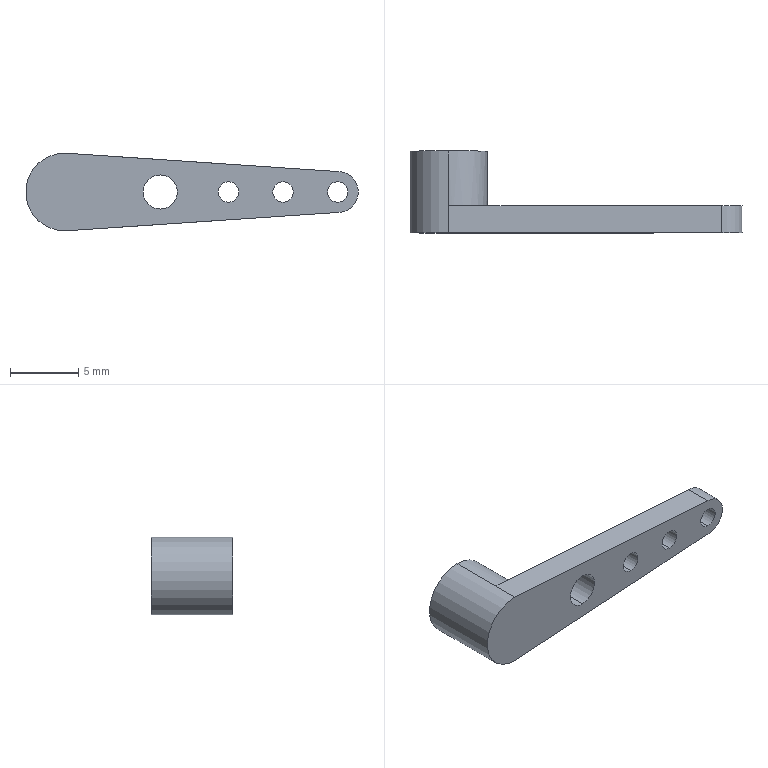Part | SolidWorks | features ICE 2, Extrusion 1 | 1 solid | 21 faces | box 24.35 x 6 x 5.701 mm | volume 238.009 mm3 | cylinder 13 | plane 8 | commonest cylinder face diameters 1.5 x6 2.5 x2 4 x2 5.701 x2 3 x1
STEP:
#1=CARTESIAN_POINT('',(20.,2.,-0.75));
#2=VERTEX_POINT('',#1);
#3=CARTESIAN_POINT('',(20.,2.,0.75));
#4=VERTEX_POINT('',#3);
#5=CARTESIAN_POINT('',(20.,2.,0.));
#6=DIRECTION('',(0.,1.,0.));
#7=DIRECTION('',(0.,0.,1.));
#8=AXIS2_PLACEMENT_3D('',#5,#6,#7);
#9=CIRCLE('',#8,0.75);
#10=EDGE_CURVE('',#2,#4,#9,.T.);
#11=ORIENTED_EDGE('',*,*,#10,.T.);
#12=CARTESIAN_POINT('',(20.,0.,0.75));
#13=VERTEX_POINT('',#12);
#14=CARTESIAN_POINT('',(20.,10.,0.75));
#15=DIRECTION('',(0.,-1.,0.));
#16=VECTOR('',#15,1000.);
#17=LINE('',#14,#16);
#18=EDGE_CURVE('',#4,#13,#17,.T.);
#19=ORIENTED_EDGE('',*,*,#18,.T.);
#20=CARTESIAN_POINT('',(20.,0.,-0.75));
#21=VERTEX_POINT('',#20);
#22=CARTESIAN_POINT('',(20.,0.,0.));
#23=DIRECTION('',(0.,-1.,0.));
#24=DIRECTION('',(0.,0.,-1.));
#25=AXIS2_PLACEMENT_3D('',#22,#23,#24);
#26=CIRCLE('',#25,0.75);
#27=EDGE_CURVE('',#13,#21,#26,.T.);
#28=ORIENTED_EDGE('',*,*,#27,.T.);
#29=CARTESIAN_POINT('',(20.,10.,-0.75));
#30=DIRECTION('',(0.,-1.,0.));
#31=VECTOR('',#30,1000.);
#32=LINE('',#29,#31);
#33=EDGE_CURVE('',#2,#21,#32,.T.);
#34=ORIENTED_EDGE('',*,*,#33,.F.);
#35=EDGE_LOOP('',(#11,#19,#28,#34));
#36=FACE_OUTER_BOUND('',#35,.T.);
#37=CARTESIAN_POINT('',(20.,10.,0.));
#38=DIRECTION('',(0.,-1.,0.));
#39=DIRECTION('',(0.,0.,-1.));
#40=AXIS2_PLACEMENT_3D('',#37,#38,#39);
#41=CYLINDRICAL_SURFACE('',#40,0.75);
#42=ADVANCED_FACE('',(#36),#41,.F.);
#43=CARTESIAN_POINT('',(7.,2.,-1.25));
#44=VERTEX_POINT('',#43);
#45=CARTESIAN_POINT('',(7.,2.,1.25));
#46=VERTEX_POINT('',#45);
#47=CARTESIAN_POINT('',(7.,2.,0.));
#48=DIRECTION('',(0.,1.,0.));
#49=DIRECTION('',(0.,0.,1.));
#50=AXIS2_PLACEMENT_3D('',#47,#48,#49);
#51=CIRCLE('',#50,1.25);
#52=EDGE_CURVE('',#44,#46,#51,.T.);
#53=ORIENTED_EDGE('',*,*,#52,.T.);
#54=CARTESIAN_POINT('',(7.,0.,1.25));
#55=VERTEX_POINT('',#54);
#56=CARTESIAN_POINT('',(7.,10.,1.25));
#57=DIRECTION('',(0.,-1.,0.));
#58=VECTOR('',#57,1000.);
#59=LINE('',#56,#58);
#60=EDGE_CURVE('',#46,#55,#59,.T.);
#61=ORIENTED_EDGE('',*,*,#60,.T.);
#62=CARTESIAN_POINT('',(7.,0.,-1.25));
#63=VERTEX_POINT('',#62);
#64=CARTESIAN_POINT('',(7.,0.,0.));
#65=DIRECTION('',(0.,-1.,0.));
#66=DIRECTION('',(0.,0.,-1.));
#67=AXIS2_PLACEMENT_3D('',#64,#65,#66);
#68=CIRCLE('',#67,1.25);
#69=EDGE_CURVE('',#55,#63,#68,.T.);
#70=ORIENTED_EDGE('',*,*,#69,.T.);
#71=CARTESIAN_POINT('',(7.,10.,-1.25));
#72=DIRECTION('',(0.,-1.,0.));
#73=VECTOR('',#72,1000.);
#74=LINE('',#71,#73);
#75=EDGE_CURVE('',#44,#63,#74,.T.);
#76=ORIENTED_EDGE('',*,*,#75,.F.);
#77=EDGE_LOOP('',(#53,#61,#70,#76));
#78=FACE_OUTER_BOUND('',#77,.T.);
#79=CARTESIAN_POINT('',(7.,10.,0.));
#80=DIRECTION('',(0.,-1.,0.));
#81=DIRECTION('',(0.,0.,-1.));
#82=AXIS2_PLACEMENT_3D('',#79,#80,#81);
#83=CYLINDRICAL_SURFACE('',#82,1.25);
#84=ADVANCED_FACE('',(#78),#83,.F.);
#85=CARTESIAN_POINT('',(12.,2.,-0.75));
#86=VERTEX_POINT('',#85);
#87=CARTESIAN_POINT('',(12.,2.,0.75));
#88=VERTEX_POINT('',#87);
#89=CARTESIAN_POINT('',(12.,2.,0.));
#90=DIRECTION('',(0.,1.,0.));
#91=DIRECTION('',(0.,0.,1.));
#92=AXIS2_PLACEMENT_3D('',#89,#90,#91);
#93=CIRCLE('',#92,0.75);
#94=EDGE_CURVE('',#86,#88,#93,.T.);
#95=ORIENTED_EDGE('',*,*,#94,.T.);
#96=CARTESIAN_POINT('',(12.,0.,0.75));
#97=VERTEX_POINT('',#96);
#98=CARTESIAN_POINT('',(12.,10.,0.75));
#99=DIRECTION('',(0.,-1.,0.));
#100=VECTOR('',#99,1000.);
#101=LINE('',#98,#100);
#102=EDGE_CURVE('',#88,#97,#101,.T.);
#103=ORIENTED_EDGE('',*,*,#102,.T.);
#104=CARTESIAN_POINT('',(12.,0.,-0.75));
#105=VERTEX_POINT('',#104);
#106=CARTESIAN_POINT('',(12.,0.,0.));
#107=DIRECTION('',(0.,-1.,0.));
#108=DIRECTION('',(0.,0.,-1.));
#109=AXIS2_PLACEMENT_3D('',#106,#107,#108);
#110=CIRCLE('',#109,0.75);
#111=EDGE_CURVE('',#97,#105,#110,.T.);
#112=ORIENTED_EDGE('',*,*,#111,.T.);
#113=CARTESIAN_POINT('',(12.,10.,-0.75));
#114=DIRECTION('',(0.,-1.,0.));
#115=VECTOR('',#114,1000.);
#116=LINE('',#113,#115);
#117=EDGE_CURVE('',#86,#105,#116,.T.);
#118=ORIENTED_EDGE('',*,*,#117,.F.);
#119=EDGE_LOOP('',(#95,#103,#112,#118));
#120=FACE_OUTER_BOUND('',#119,.T.);
#121=CARTESIAN_POINT('',(12.,10.,0.));
#122=DIRECTION('',(0.,-1.,0.));
#123=DIRECTION('',(0.,0.,-1.));
#124=AXIS2_PLACEMENT_3D('',#121,#122,#123);
#125=CYLINDRICAL_SURFACE('',#124,0.75);
#126=ADVANCED_FACE('',(#120),#125,.F.);
#127=CARTESIAN_POINT('',(16.,2.,-0.75));
#128=VERTEX_POINT('',#127);
#129=CARTESIAN_POINT('',(16.,2.,0.75));
#130=VERTEX_POINT('',#129);
#131=CARTESIAN_POINT('',(16.,2.,0.));
#132=DIRECTION('',(0.,1.,0.));
#133=DIRECTION('',(0.,0.,1.));
#134=AXIS2_PLACEMENT_3D('',#131,#132,#133);
#135=CIRCLE('',#134,0.75);
#136=EDGE_CURVE('',#128,#130,#135,.T.);
#137=ORIENTED_EDGE('',*,*,#136,.T.);
#138=CARTESIAN_POINT('',(16.,0.,0.75));
#139=VERTEX_POINT('',#138);
#140=CARTESIAN_POINT('',(16.,10.,0.75));
#141=DIRECTION('',(0.,-1.,0.));
#142=VECTOR('',#141,1000.);
#143=LINE('',#140,#142);
#144=EDGE_CURVE('',#130,#139,#143,.T.);
#145=ORIENTED_EDGE('',*,*,#144,.T.);
#146=CARTESIAN_POINT('',(16.,0.,-0.75));
#147=VERTEX_POINT('',#146);
#148=CARTESIAN_POINT('',(16.,0.,0.));
#149=DIRECTION('',(0.,-1.,0.));
#150=DIRECTION('',(0.,0.,-1.));
#151=AXIS2_PLACEMENT_3D('',#148,#149,#150);
#152=CIRCLE('',#151,0.75);
#153=EDGE_CURVE('',#139,#147,#152,.T.);
#154=ORIENTED_EDGE('',*,*,#153,.T.);
#155=CARTESIAN_POINT('',(16.,10.,-0.75));
#156=DIRECTION('',(0.,-1.,0.));
#157=VECTOR('',#156,1000.);
#158=LINE('',#155,#157);
#159=EDGE_CURVE('',#128,#147,#158,.T.);
#160=ORIENTED_EDGE('',*,*,#159,.F.);
#161=EDGE_LOOP('',(#137,#145,#154,#160));
#162=FACE_OUTER_BOUND('',#161,.T.);
#163=CARTESIAN_POINT('',(16.,10.,0.));
#164=DIRECTION('',(0.,-1.,0.));
#165=DIRECTION('',(0.,0.,-1.));
#166=AXIS2_PLACEMENT_3D('',#163,#164,#165);
#167=CYLINDRICAL_SURFACE('',#166,0.75);
#168=ADVANCED_FACE('',(#162),#167,.F.);
#169=CARTESIAN_POINT('',(0.,6.,-2.));
#170=VERTEX_POINT('',#169);
#171=CARTESIAN_POINT('',(0.,6.,2.));
#172=VERTEX_POINT('',#171);
#173=CARTESIAN_POINT('',(0.,6.,0.));
#174=DIRECTION('',(0.,1.,0.));
#175=DIRECTION('',(0.,0.,1.));
#176=AXIS2_PLACEMENT_3D('',#173,#174,#175);
#177=CIRCLE('',#176,2.);
#178=EDGE_CURVE('',#170,#172,#177,.T.);
#179=ORIENTED_EDGE('',*,*,#178,.T.);
#180=CARTESIAN_POINT('',(0.,2.,2.));
#181=VERTEX_POINT('',#180);
#182=CARTESIAN_POINT('',(0.,6.,2.));
#183=DIRECTION('',(0.,-1.,0.));
#184=VECTOR('',#183,1000.);
#185=LINE('',#182,#184);
#186=EDGE_CURVE('',#172,#181,#185,.T.);
#187=ORIENTED_EDGE('',*,*,#186,.T.);
#188=CARTESIAN_POINT('',(0.,2.,-2.));
#189=VERTEX_POINT('',#188);
#190=CARTESIAN_POINT('',(0.,2.,0.));
#191=DIRECTION('',(0.,1.,0.));
#192=DIRECTION('',(0.,0.,1.));
#193=AXIS2_PLACEMENT_3D('',#190,#191,#192);
#194=CIRCLE('',#193,2.);
#195=EDGE_CURVE('',#189,#181,#194,.T.);
#196=ORIENTED_EDGE('',*,*,#195,.F.);
#197=CARTESIAN_POINT('',(0.,6.,-2.));
#198=DIRECTION('',(0.,-1.,0.));
#199=VECTOR('',#198,1000.);
#200=LINE('',#197,#199);
#201=EDGE_CURVE('',#170,#189,#200,.T.);
#202=ORIENTED_EDGE('',*,*,#201,.F.);
#203=EDGE_LOOP('',(#179,#187,#196,#202));
#204=FACE_OUTER_BOUND('',#203,.T.);
#205=CARTESIAN_POINT('',(0.,6.,0.));
#206=DIRECTION('',(0.,-1.,0.));
#207=DIRECTION('',(0.,0.,-1.));
#208=AXIS2_PLACEMENT_3D('',#205,#206,#207);
#209=CYLINDRICAL_SURFACE('',#208,2.);
#210=ADVANCED_FACE('',(#204),#209,.F.);
#211=CARTESIAN_POINT('',(0.,6.,2.85));
#212=VERTEX_POINT('',#211);
#213=CARTESIAN_POINT('',(0.,6.,-2.85));
#214=VERTEX_POINT('',#213);
#215=CARTESIAN_POINT('',(0.,6.,0.));
#216=DIRECTION('',(0.,1.,0.));
#217=DIRECTION('',(0.,0.,1.));
#218=AXIS2_PLACEMENT_3D('',#215,#216,#217);
#219=CIRCLE('',#218,2.85);
#220=EDGE_CURVE('',#212,#214,#219,.T.);
#221=ORIENTED_EDGE('',*,*,#220,.F.);
#222=CARTESIAN_POINT('',(0.,2.,2.85));
#223=VERTEX_POINT('',#222);
#224=CARTESIAN_POINT('',(0.,2.,2.85));
#225=DIRECTION('',(0.,-1.,0.));
#226=VECTOR('',#225,1000.);
#227=LINE('',#224,#226);
#228=EDGE_CURVE('',#212,#223,#227,.T.);
#229=ORIENTED_EDGE('',*,*,#228,.T.);
#230=CARTESIAN_POINT('',(0.3831,2.,2.824));
#231=VERTEX_POINT('',#230);
#232=CARTESIAN_POINT('',(0.,2.,0.));
#233=DIRECTION('',(0.,1.,0.));
#234=DIRECTION('',(0.,0.,1.));
#235=AXIS2_PLACEMENT_3D('',#232,#233,#234);
#236=CIRCLE('',#235,2.85);
#237=EDGE_CURVE('',#223,#231,#236,.T.);
#238=ORIENTED_EDGE('',*,*,#237,.T.);
#239=CARTESIAN_POINT('',(0.3831,2.,-2.824));
#240=VERTEX_POINT('',#239);
#241=CARTESIAN_POINT('',(0.,2.,0.));
#242=DIRECTION('',(0.,1.,0.));
#243=DIRECTION('',(0.,0.,1.));
#244=AXIS2_PLACEMENT_3D('',#241,#242,#243);
#245=CIRCLE('',#244,2.85);
#246=EDGE_CURVE('',#231,#240,#245,.T.);
#247=ORIENTED_EDGE('',*,*,#246,.T.);
#248=CARTESIAN_POINT('',(0.,2.,-2.85));
#249=VERTEX_POINT('',#248);
#250=CARTESIAN_POINT('',(0.,2.,0.));
#251=DIRECTION('',(0.,1.,0.));
#252=DIRECTION('',(0.,0.,1.));
#253=AXIS2_PLACEMENT_3D('',#250,#251,#252);
#254=CIRCLE('',#253,2.85);
#255=EDGE_CURVE('',#240,#249,#254,.T.);
#256=ORIENTED_EDGE('',*,*,#255,.T.);
#257=CARTESIAN_POINT('',(0.,2.,-2.85));
#258=DIRECTION('',(0.,-1.,0.));
#259=VECTOR('',#258,1000.);
#260=LINE('',#257,#259);
#261=EDGE_CURVE('',#214,#249,#260,.T.);
#262=ORIENTED_EDGE('',*,*,#261,.F.);
#263=EDGE_LOOP('',(#221,#229,#238,#247,#256,#262));
#264=FACE_OUTER_BOUND('',#263,.T.);
#265=CARTESIAN_POINT('',(0.,2.,0.));
#266=DIRECTION('',(0.,-1.,0.));
#267=DIRECTION('',(0.,0.,-1.));
#268=AXIS2_PLACEMENT_3D('',#265,#266,#267);
#269=CYLINDRICAL_SURFACE('',#268,2.85);
#270=ADVANCED_FACE('',(#264),#269,.T.);
#271=ORIENTED_EDGE('',*,*,#228,.F.);
#272=CARTESIAN_POINT('',(0.,6.,0.));
#273=DIRECTION('',(0.,1.,0.));
#274=DIRECTION('',(0.,0.,1.));
#275=AXIS2_PLACEMENT_3D('',#272,#273,#274);
#276=CIRCLE('',#275,2.85);
#277=EDGE_CURVE('',#214,#212,#276,.T.);
#278=ORIENTED_EDGE('',*,*,#277,.F.);
#279=ORIENTED_EDGE('',*,*,#261,.T.);
#280=CARTESIAN_POINT('',(0.,0.,-2.85));
#281=VERTEX_POINT('',#280);
#282=CARTESIAN_POINT('',(0.,2.,-2.85));
#283=DIRECTION('',(0.,-1.,0.));
#284=VECTOR('',#283,1000.);
#285=LINE('',#282,#284);
#286=EDGE_CURVE('',#249,#281,#285,.T.);
#287=ORIENTED_EDGE('',*,*,#286,.T.);
#288=CARTESIAN_POINT('',(0.,0.,2.85));
#289=VERTEX_POINT('',#288);
#290=CARTESIAN_POINT('',(0.,0.,0.));
#291=DIRECTION('',(0.,1.,0.));
#292=DIRECTION('',(0.,0.,1.));
#293=AXIS2_PLACEMENT_3D('',#290,#291,#292);
#294=CIRCLE('',#293,2.85);
#295=EDGE_CURVE('',#281,#289,#294,.T.);
#296=ORIENTED_EDGE('',*,*,#295,.T.);
#297=CARTESIAN_POINT('',(0.,2.,2.85));
#298=DIRECTION('',(0.,-1.,0.));
#299=VECTOR('',#298,1000.);
#300=LINE('',#297,#299);
#301=EDGE_CURVE('',#223,#289,#300,.T.);
#302=ORIENTED_EDGE('',*,*,#301,.F.);
#303=EDGE_LOOP('',(#271,#278,#279,#287,#296,#302));
#304=FACE_OUTER_BOUND('',#303,.T.);
#305=CARTESIAN_POINT('',(0.,2.,0.));
#306=DIRECTION('',(0.,-1.,0.));
#307=DIRECTION('',(0.,0.,-1.));
#308=AXIS2_PLACEMENT_3D('',#305,#306,#307);
#309=CYLINDRICAL_SURFACE('',#308,2.85);
#310=ADVANCED_FACE('',(#304),#309,.T.);
#311=CARTESIAN_POINT('',(20.,0.,1.5));
#312=VERTEX_POINT('',#311);
#313=CARTESIAN_POINT('',(0.,0.,2.85));
#314=DIRECTION('',(0.9977,0.,-0.06736));
#315=VECTOR('',#314,1000.);
#316=LINE('',#313,#315);
#317=EDGE_CURVE('',#289,#312,#316,.T.);
#318=ORIENTED_EDGE('',*,*,#317,.T.);
#319=CARTESIAN_POINT('',(20.,2.,1.5));
#320=VERTEX_POINT('',#319);
#321=CARTESIAN_POINT('',(20.,2.,1.5));
#322=DIRECTION('',(0.,-1.,0.));
#323=VECTOR('',#322,1000.);
#324=LINE('',#321,#323);
#325=EDGE_CURVE('',#320,#312,#324,.T.);
#326=ORIENTED_EDGE('',*,*,#325,.F.);
#327=CARTESIAN_POINT('',(0.,2.,2.85));
#328=DIRECTION('',(0.9977,0.,-0.06736));
#329=VECTOR('',#328,1000.);
#330=LINE('',#327,#329);
#331=EDGE_CURVE('',#231,#320,#330,.T.);
#332=ORIENTED_EDGE('',*,*,#331,.F.);
#333=CARTESIAN_POINT('',(0.,2.,2.85));
#334=DIRECTION('',(0.9977,0.,-0.06736));
#335=VECTOR('',#334,1000.);
#336=LINE('',#333,#335);
#337=EDGE_CURVE('',#223,#231,#336,.T.);
#338=ORIENTED_EDGE('',*,*,#337,.F.);
#339=ORIENTED_EDGE('',*,*,#301,.T.);
#340=EDGE_LOOP('',(#318,#326,#332,#338,#339));
#341=FACE_OUTER_BOUND('',#340,.T.);
#342=CARTESIAN_POINT('',(0.,2.,2.85));
#343=DIRECTION('',(-0.06736,0.,-0.9977));
#344=DIRECTION('',(-0.9977,0.,0.06736));
#345=AXIS2_PLACEMENT_3D('',#342,#343,#344);
#346=PLANE('',#345);
#347=ADVANCED_FACE('',(#341),#346,.F.);
#348=CARTESIAN_POINT('',(20.,0.,-1.5));
#349=VERTEX_POINT('',#348);
#350=CARTESIAN_POINT('',(20.,0.,0.));
#351=DIRECTION('',(0.,1.,0.));
#352=DIRECTION('',(0.,0.,1.));
#353=AXIS2_PLACEMENT_3D('',#350,#351,#352);
#354=CIRCLE('',#353,1.5);
#355=EDGE_CURVE('',#312,#349,#354,.T.);
#356=ORIENTED_EDGE('',*,*,#355,.T.);
#357=CARTESIAN_POINT('',(20.,2.,-1.5));
#358=VERTEX_POINT('',#357);
#359=CARTESIAN_POINT('',(20.,2.,-1.5));
#360=DIRECTION('',(0.,-1.,0.));
#361=VECTOR('',#360,1000.);
#362=LINE('',#359,#361);
#363=EDGE_CURVE('',#358,#349,#362,.T.);
#364=ORIENTED_EDGE('',*,*,#363,.F.);
#365=CARTESIAN_POINT('',(20.,2.,0.));
#366=DIRECTION('',(0.,1.,0.));
#367=DIRECTION('',(0.,0.,1.));
#368=AXIS2_PLACEMENT_3D('',#365,#366,#367);
#369=CIRCLE('',#368,1.5);
#370=EDGE_CURVE('',#320,#358,#369,.T.);
#371=ORIENTED_EDGE('',*,*,#370,.F.);
#372=ORIENTED_EDGE('',*,*,#325,.T.);
#373=EDGE_LOOP('',(#356,#364,#371,#372));
#374=FACE_OUTER_BOUND('',#373,.T.);
#375=CARTESIAN_POINT('',(20.,2.,0.));
#376=DIRECTION('',(0.,-1.,0.));
#377=DIRECTION('',(0.,0.,-1.));
#378=AXIS2_PLACEMENT_3D('',#375,#376,#377);
#379=CYLINDRICAL_SURFACE('',#378,1.5);
#380=ADVANCED_FACE('',(#374),#379,.T.);
#381=CARTESIAN_POINT('',(0.,0.,-2.85));
#382=DIRECTION('',(-0.9977,0.,-0.06736));
#383=VECTOR('',#382,1000.);
#384=LINE('',#381,#383);
#385=EDGE_CURVE('',#349,#281,#384,.T.);
#386=ORIENTED_EDGE('',*,*,#385,.T.);
#387=ORIENTED_EDGE('',*,*,#286,.F.);
#388=CARTESIAN_POINT('',(0.,2.,-2.85));
#389=DIRECTION('',(-0.9977,0.,-0.06736));
#390=VECTOR('',#389,1000.);
#391=LINE('',#388,#390);
#392=EDGE_CURVE('',#240,#249,#391,.T.);
#393=ORIENTED_EDGE('',*,*,#392,.F.);
#394=CARTESIAN_POINT('',(0.,2.,-2.85));
#395=DIRECTION('',(-0.9977,0.,-0.06736));
#396=VECTOR('',#395,1000.);
#397=LINE('',#394,#396);
#398=EDGE_CURVE('',#358,#240,#397,.T.);
#399=ORIENTED_EDGE('',*,*,#398,.F.);
#400=ORIENTED_EDGE('',*,*,#363,.T.);
#401=EDGE_LOOP('',(#386,#387,#393,#399,#400));
#402=FACE_OUTER_BOUND('',#401,.T.);
#403=CARTESIAN_POINT('',(0.,2.,-2.85));
#404=DIRECTION('',(-0.06736,0.,0.9977));
#405=DIRECTION('',(0.9977,0.,0.06736));
#406=AXIS2_PLACEMENT_3D('',#403,#404,#405);
#407=PLANE('',#406);
#408=ADVANCED_FACE('',(#402),#407,.F.);
#409=ORIENTED_EDGE('',*,*,#10,.F.);
#410=CARTESIAN_POINT('',(20.,2.,0.));
#411=DIRECTION('',(0.,1.,0.));
#412=DIRECTION('',(0.,0.,1.));
#413=AXIS2_PLACEMENT_3D('',#410,#411,#412);
#414=CIRCLE('',#413,0.75);
#415=EDGE_CURVE('',#4,#2,#414,.T.);
#416=ORIENTED_EDGE('',*,*,#415,.F.);
#417=EDGE_LOOP('',(#409,#416));
#418=FACE_BOUND('',#417,.T.);
#419=ORIENTED_EDGE('',*,*,#52,.F.);
#420=CARTESIAN_POINT('',(7.,2.,0.));
#421=DIRECTION('',(0.,1.,0.));
#422=DIRECTION('',(0.,0.,1.));
#423=AXIS2_PLACEMENT_3D('',#420,#421,#422);
#424=CIRCLE('',#423,1.25);
#425=EDGE_CURVE('',#46,#44,#424,.T.);
#426=ORIENTED_EDGE('',*,*,#425,.F.);
#427=EDGE_LOOP('',(#419,#426));
#428=FACE_BOUND('',#427,.T.);
#429=ORIENTED_EDGE('',*,*,#94,.F.);
#430=CARTESIAN_POINT('',(12.,2.,0.));
#431=DIRECTION('',(0.,1.,0.));
#432=DIRECTION('',(0.,0.,1.));
#433=AXIS2_PLACEMENT_3D('',#430,#431,#432);
#434=CIRCLE('',#433,0.75);
#435=EDGE_CURVE('',#88,#86,#434,.T.);
#436=ORIENTED_EDGE('',*,*,#435,.F.);
#437=EDGE_LOOP('',(#429,#436));
#438=FACE_BOUND('',#437,.T.);
#439=ORIENTED_EDGE('',*,*,#136,.F.);
#440=CARTESIAN_POINT('',(16.,2.,0.));
#441=DIRECTION('',(0.,1.,0.));
#442=DIRECTION('',(0.,0.,1.));
#443=AXIS2_PLACEMENT_3D('',#440,#441,#442);
#444=CIRCLE('',#443,0.75);
#445=EDGE_CURVE('',#130,#128,#444,.T.);
#446=ORIENTED_EDGE('',*,*,#445,.F.);
#447=EDGE_LOOP('',(#439,#446));
#448=FACE_BOUND('',#447,.T.);
#449=ORIENTED_EDGE('',*,*,#246,.F.);
#450=ORIENTED_EDGE('',*,*,#331,.T.);
#451=ORIENTED_EDGE('',*,*,#370,.T.);
#452=ORIENTED_EDGE('',*,*,#398,.T.);
#453=EDGE_LOOP('',(#449,#450,#451,#452));
#454=FACE_OUTER_BOUND('',#453,.T.);
#455=CARTESIAN_POINT('',(0.,2.,0.));
#456=DIRECTION('',(0.,1.,0.));
#457=DIRECTION('',(0.,0.,1.));
#458=AXIS2_PLACEMENT_3D('',#455,#456,#457);
#459=PLANE('',#458);
#460=ADVANCED_FACE('',(#418,#428,#438,#448,#454),#459,.T.);
#461=CARTESIAN_POINT('',(20.,0.,0.));
#462=DIRECTION('',(0.,-1.,0.));
#463=DIRECTION('',(0.,0.,-1.));
#464=AXIS2_PLACEMENT_3D('',#461,#462,#463);
#465=CIRCLE('',#464,0.75);
#466=EDGE_CURVE('',#21,#13,#465,.T.);
#467=ORIENTED_EDGE('',*,*,#466,.F.);
#468=ORIENTED_EDGE('',*,*,#27,.F.);
#469=EDGE_LOOP('',(#467,#468));
#470=FACE_BOUND('',#469,.T.);
#471=CARTESIAN_POINT('',(7.,0.,0.));
#472=DIRECTION('',(0.,-1.,0.));
#473=DIRECTION('',(0.,0.,-1.));
#474=AXIS2_PLACEMENT_3D('',#471,#472,#473);
#475=CIRCLE('',#474,1.25);
#476=EDGE_CURVE('',#63,#55,#475,.T.);
#477=ORIENTED_EDGE('',*,*,#476,.F.);
#478=ORIENTED_EDGE('',*,*,#69,.F.);
#479=EDGE_LOOP('',(#477,#478));
#480=FACE_BOUND('',#479,.T.);
#481=CARTESIAN_POINT('',(12.,0.,0.));
#482=DIRECTION('',(0.,-1.,0.));
#483=DIRECTION('',(0.,0.,-1.));
#484=AXIS2_PLACEMENT_3D('',#481,#482,#483);
#485=CIRCLE('',#484,0.75);
#486=EDGE_CURVE('',#105,#97,#485,.T.);
#487=ORIENTED_EDGE('',*,*,#486,.F.);
#488=ORIENTED_EDGE('',*,*,#111,.F.);
#489=EDGE_LOOP('',(#487,#488));
#490=FACE_BOUND('',#489,.T.);
#491=CARTESIAN_POINT('',(16.,0.,0.));
#492=DIRECTION('',(0.,-1.,0.));
#493=DIRECTION('',(0.,0.,-1.));
#494=AXIS2_PLACEMENT_3D('',#491,#492,#493);
#495=CIRCLE('',#494,0.75);
#496=EDGE_CURVE('',#147,#139,#495,.T.);
#497=ORIENTED_EDGE('',*,*,#496,.F.);
#498=ORIENTED_EDGE('',*,*,#153,.F.);
#499=EDGE_LOOP('',(#497,#498));
#500=FACE_BOUND('',#499,.T.);
#501=ORIENTED_EDGE('',*,*,#295,.F.);
#502=ORIENTED_EDGE('',*,*,#385,.F.);
#503=ORIENTED_EDGE('',*,*,#355,.F.);
#504=ORIENTED_EDGE('',*,*,#317,.F.);
#505=EDGE_LOOP('',(#501,#502,#503,#504));
#506=FACE_OUTER_BOUND('',#505,.T.);
#507=CARTESIAN_POINT('',(0.,0.,0.));
#508=DIRECTION('',(0.,1.,0.));
#509=DIRECTION('',(0.,0.,1.));
#510=AXIS2_PLACEMENT_3D('',#507,#508,#509);
#511=PLANE('',#510);
#512=ADVANCED_FACE('',(#470,#480,#490,#500,#506),#511,.F.);
#513=ORIENTED_EDGE('',*,*,#237,.F.);
#514=ORIENTED_EDGE('',*,*,#337,.T.);
#515=EDGE_LOOP('',(#513,#514));
#516=FACE_OUTER_BOUND('',#515,.T.);
#517=CARTESIAN_POINT('',(0.,2.,0.));
#518=DIRECTION('',(0.,1.,0.));
#519=DIRECTION('',(0.,0.,1.));
#520=AXIS2_PLACEMENT_3D('',#517,#518,#519);
#521=PLANE('',#520);
#522=ADVANCED_FACE('',(#516),#521,.F.);
#523=ORIENTED_EDGE('',*,*,#255,.F.);
#524=ORIENTED_EDGE('',*,*,#392,.T.);
#525=EDGE_LOOP('',(#523,#524));
#526=FACE_OUTER_BOUND('',#525,.T.);
#527=CARTESIAN_POINT('',(0.,2.,0.));
#528=DIRECTION('',(0.,1.,0.));
#529=DIRECTION('',(0.,0.,1.));
#530=AXIS2_PLACEMENT_3D('',#527,#528,#529);
#531=PLANE('',#530);
#532=ADVANCED_FACE('',(#526),#531,.F.);
#533=ORIENTED_EDGE('',*,*,#277,.T.);
#534=ORIENTED_EDGE('',*,*,#220,.T.);
#535=EDGE_LOOP('',(#533,#534));
#536=FACE_OUTER_BOUND('',#535,.T.);
#537=ORIENTED_EDGE('',*,*,#178,.F.);
#538=CARTESIAN_POINT('',(0.,6.,0.));
#539=DIRECTION('',(0.,1.,0.));
#540=DIRECTION('',(0.,0.,1.));
#541=AXIS2_PLACEMENT_3D('',#538,#539,#540);
#542=CIRCLE('',#541,2.);
#543=EDGE_CURVE('',#172,#170,#542,.T.);
#544=ORIENTED_EDGE('',*,*,#543,.F.);
#545=EDGE_LOOP('',(#537,#544));
#546=FACE_BOUND('',#545,.T.);
#547=CARTESIAN_POINT('',(0.,6.,0.));
#548=DIRECTION('',(0.,1.,0.));
#549=DIRECTION('',(0.,0.,1.));
#550=AXIS2_PLACEMENT_3D('',#547,#548,#549);
#551=PLANE('',#550);
#552=ADVANCED_FACE('',(#536,#546),#551,.T.);
#553=ORIENTED_EDGE('',*,*,#186,.F.);
#554=ORIENTED_EDGE('',*,*,#543,.T.);
#555=ORIENTED_EDGE('',*,*,#201,.T.);
#556=CARTESIAN_POINT('',(0.,2.,0.));
#557=DIRECTION('',(0.,1.,0.));
#558=DIRECTION('',(0.,0.,1.));
#559=AXIS2_PLACEMENT_3D('',#556,#557,#558);
#560=CIRCLE('',#559,2.);
#561=EDGE_CURVE('',#181,#189,#560,.T.);
#562=ORIENTED_EDGE('',*,*,#561,.F.);
#563=EDGE_LOOP('',(#553,#554,#555,#562));
#564=FACE_OUTER_BOUND('',#563,.T.);
#565=CARTESIAN_POINT('',(0.,6.,0.));
#566=DIRECTION('',(0.,-1.,0.));
#567=DIRECTION('',(0.,0.,-1.));
#568=AXIS2_PLACEMENT_3D('',#565,#566,#567);
#569=CYLINDRICAL_SURFACE('',#568,2.);
#570=ADVANCED_FACE('',(#564),#569,.F.);
#571=ORIENTED_EDGE('',*,*,#195,.T.);
#572=ORIENTED_EDGE('',*,*,#561,.T.);
#573=EDGE_LOOP('',(#571,#572));
#574=FACE_OUTER_BOUND('',#573,.T.);
#575=CARTESIAN_POINT('',(0.,2.,0.));
#576=DIRECTION('',(0.,1.,0.));
#577=DIRECTION('',(0.,0.,1.));
#578=AXIS2_PLACEMENT_3D('',#575,#576,#577);
#579=PLANE('',#578);
#580=ADVANCED_FACE('',(#574),#579,.T.);
#581=ORIENTED_EDGE('',*,*,#144,.F.);
#582=ORIENTED_EDGE('',*,*,#445,.T.);
#583=ORIENTED_EDGE('',*,*,#159,.T.);
#584=ORIENTED_EDGE('',*,*,#496,.T.);
#585=EDGE_LOOP('',(#581,#582,#583,#584));
#586=FACE_OUTER_BOUND('',#585,.T.);
#587=CARTESIAN_POINT('',(16.,10.,0.));
#588=DIRECTION('',(0.,-1.,0.));
#589=DIRECTION('',(0.,0.,-1.));
#590=AXIS2_PLACEMENT_3D('',#587,#588,#589);
#591=CYLINDRICAL_SURFACE('',#590,0.75);
#592=ADVANCED_FACE('',(#586),#591,.F.);
#593=ORIENTED_EDGE('',*,*,#102,.F.);
#594=ORIENTED_EDGE('',*,*,#435,.T.);
#595=ORIENTED_EDGE('',*,*,#117,.T.);
#596=ORIENTED_EDGE('',*,*,#486,.T.);
#597=EDGE_LOOP('',(#593,#594,#595,#596));
#598=FACE_OUTER_BOUND('',#597,.T.);
#599=CARTESIAN_POINT('',(12.,10.,0.));
#600=DIRECTION('',(0.,-1.,0.));
#601=DIRECTION('',(0.,0.,-1.));
#602=AXIS2_PLACEMENT_3D('',#599,#600,#601);
#603=CYLINDRICAL_SURFACE('',#602,0.75);
#604=ADVANCED_FACE('',(#598),#603,.F.);
#605=ORIENTED_EDGE('',*,*,#60,.F.);
#606=ORIENTED_EDGE('',*,*,#425,.T.);
#607=ORIENTED_EDGE('',*,*,#75,.T.);
#608=ORIENTED_EDGE('',*,*,#476,.T.);
#609=EDGE_LOOP('',(#605,#606,#607,#608));
#610=FACE_OUTER_BOUND('',#609,.T.);
#611=CARTESIAN_POINT('',(7.,10.,0.));
#612=DIRECTION('',(0.,-1.,0.));
#613=DIRECTION('',(0.,0.,-1.));
#614=AXIS2_PLACEMENT_3D('',#611,#612,#613);
#615=CYLINDRICAL_SURFACE('',#614,1.25);
#616=ADVANCED_FACE('',(#610),#615,.F.);
#617=ORIENTED_EDGE('',*,*,#18,.F.);
#618=ORIENTED_EDGE('',*,*,#415,.T.);
#619=ORIENTED_EDGE('',*,*,#33,.T.);
#620=ORIENTED_EDGE('',*,*,#466,.T.);
#621=EDGE_LOOP('',(#617,#618,#619,#620));
#622=FACE_OUTER_BOUND('',#621,.T.);
#623=CARTESIAN_POINT('',(20.,10.,0.));
#624=DIRECTION('',(0.,-1.,0.));
#625=DIRECTION('',(0.,0.,-1.));
#626=AXIS2_PLACEMENT_3D('',#623,#624,#625);
#627=CYLINDRICAL_SURFACE('',#626,0.75);
#628=ADVANCED_FACE('',(#622),#627,.F.);
#629=CLOSED_SHELL('',(#42,#84,#126,#168,#210,#270,#310,#347,#380,#408,#460,#512,#522,#532,#552,#570,#580,#592,#604,#616,#628));
#630=MANIFOLD_SOLID_BREP('',#629);
#631=CARTESIAN_POINT('',(0.,0.,0.));
#632=DIRECTION('',(0.,0.,1.));
#633=DIRECTION('',(1.,0.,0.));
#634=AXIS2_PLACEMENT_3D('',#631,#632,#633);
#635=(LENGTH_UNIT()NAMED_UNIT(*)SI_UNIT(.MILLI.,.METRE.));
#636=UNCERTAINTY_MEASURE_WITH_UNIT(LENGTH_MEASURE(0.00001),#635,'','');
#637=(NAMED_UNIT(*)PLANE_ANGLE_UNIT()SI_UNIT($,.RADIAN.));
#638=(NAMED_UNIT(*)SI_UNIT($,.STERADIAN.)SOLID_ANGLE_UNIT());
#639=(GEOMETRIC_REPRESENTATION_CONTEXT(3)GLOBAL_UNCERTAINTY_ASSIGNED_CONTEXT((#636))GLOBAL_UNIT_ASSIGNED_CONTEXT((#635,#637,#638))REPRESENTATION_CONTEXT('',''));
#640=ADVANCED_BREP_SHAPE_REPRESENTATION('',(#630,#634),#639);